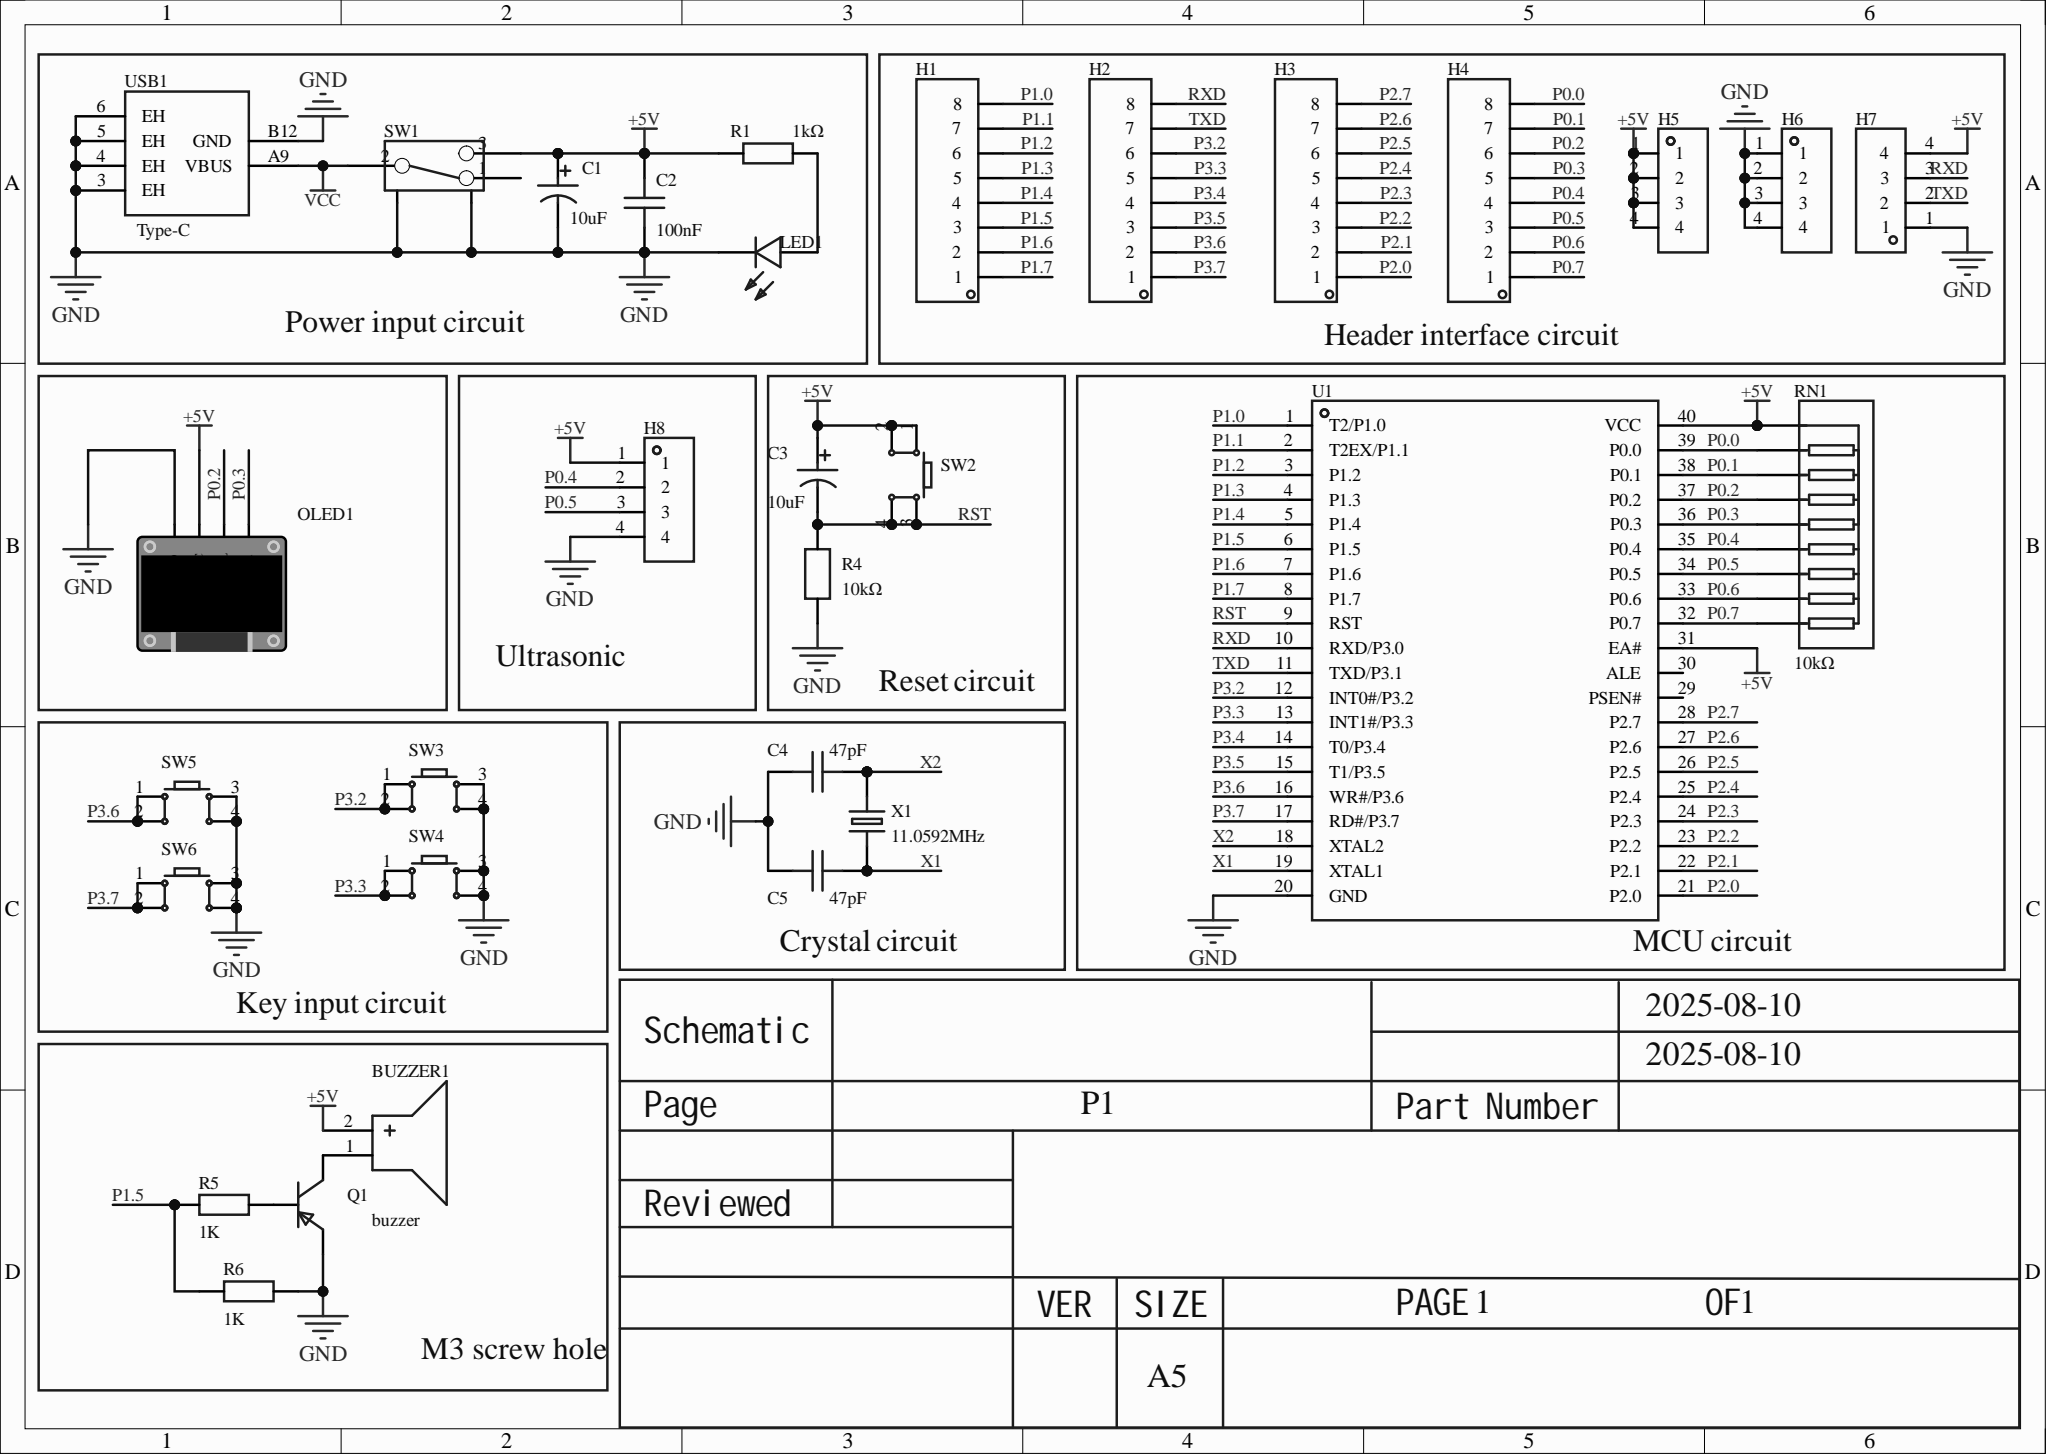Circuit board | Altium Designer | 47 parts | 49 nets
Bill of materials:
Comment,Description,Designator,Footprint,LibRef,Quantity
"buzzer","","BUZZER1","BUZ-TH_BD12.0-P6.00-D0.9-RD","buzzer","1"
"10uF","Capacitance: 10uF; Tolerance: ±20%; Rated voltage: 50V; Body diameter: 5mm; Body length: 11mm; Lead pitch: 2mm; Operating life: 1000hrs@105℃;","C1, C3","CAP-TH_BD5.0-P2.00-D0.8-FD","KM106M050D11RR0VH2FP0","2"
"100nF","Capacitance: 100nF; Tolerance: ±10%; Rated voltage: 50V; Temperature coefficient: X7R;","C2","CAP-TH_L8.5-W5.0-P5.00-D1.2","CT4-0805B104K500F3","1"
"47pF","Capacitance: 47pF; Tolerance: ±5%; Rated voltage: 50V; Temperature coefficient: NP0; Lead pitch: 5.08mm; Body diameter: 4.7mm; Body thickness: 2.2mm;","C4, C5","CAP-TH_L4.5-W3.0-P5.00-D1.2","CC1H470JC74DCH4B10MN","2"
"","","H1, H2, H3, H4","HDR-TH_8P-P2.54-V-M","HDR-M_2.54_1x8P","4"
"","","H5, H6, H7","HDR-TH_4P-P2.54-V-M","HDR-M_2.54_1x4P","3"
"","","H8","HDR-TH_4P-P2.54-V-F","HDR-F_2.54_1x4P","1"
"204-10SURD/S530-A3-L","Emitted color: Red; Diode configuration: -; Lens color: Diffused red; Dominant wavelength: 624nm; Peak wavelength: 632nm; Color temperature: -; Test current: 20mA; Power: 60mW; Viewing angle: 40°; Mounting style: -; Operating temperature: -40℃~+85℃;","LED1","LED-TH_BD3.0-P2.54-FD","204-10SURD/S530-A3-L","1"
"204-10SYGD/S530-E3","Emitted color: Green/Yellow-green;","LED2, LED3, LED4, LED5, LED6, LED7, LED8, LED9","LED-TH_BD3.8-P2.54-FD","204-10SYGD/S530-E3","8"
"","","OLED1","0.96OLED_4P","0.96OLED模块_4P","1"
"","","Q1","S8550P_SOT","S8550_SOT_PNP","1"
"1kΩ","Resistor type: Metal film resistor; Resistance: 1kΩ; Tolerance: ±1%; Power: 250mW; Temperature coefficient: ±50ppm/?;","R1, R2, R3, R7, R8, R9, R10, R11, R12","RES-TH_BD2.5-L6.5-P10.50-D0.6","MFR0W4F1001A50","9"
"10kΩ","","R4","RES-TH_BD2.4-L6.3-P10.30-D0.6","RN1/4W10KFT/BA1","1"
"1K","","R5, R6","R0603","Res_0603","2"
"10kΩ","Resistance: 10kΩ; Tolerance: ±5%; Power per element: 125mW; Temperature coefficient: ±100ppm/?; Resistor count: 8; Pin count: 9;","RN1","RES-ARRAY-TH_9P-P2.54-D1.0","A09-103JP","1"
"SS-12D02-VG4","Rated current (DC): -; Rated voltage (DC): -; Rated current (AC): -; Rated voltage (AC): -; Circuit configuration: SPDT; Mounting style: Through-hole; Mechanical life: 5000; Actuator shape: Rectangular post; Pin style: PC pin; Operating temperature: -25℃~+70℃; Switch height: 8.7mm;","SW1","SW-TH_SS-12D02-VG4","SS-12D02-VG4_C136719","1"
"","","SW2, SW3, SW4, SW5, SW6","SW-TH_4P-L6.0-W6.0-P4.50-LS6.5","Key_TH_6x6x6","5"
"STC89C52RC-40I-PDIP40","CPU core: 51 series; Max CPU frequency: -; Operating voltage: 3.3V~5.5V; Internal oscillator: -; External clock frequency range: -; Program FLASH size: 8KB; Total RAM: 512Byte; EEPROM/data FLASH size: 4KB; GPIO count: 35; ADC (units/channels/bits): -; DAC (units/channels/bits): -; (E)PWM (units/channels/bits): -; 8-bit Timer count: -; 16-bit Timer count: 3; 32-bit Timer count: -; Internal comparator count: -; U(S)ART count: 1; I2C count: -; I2S count: -;","U1","DIP-40_L52.0-W13.7-P2.54-LS15.2-BL","STC89C52RC-40I-PDIP40","1"
"TYPE-C-31-M-33","Connector type: Type-C; Standard: -; Gender: Female; Contact count: 2; Port count: 1; Mounting style: Right angle; Rated current - power: 3A; Operating temperature range: -30℃~+80℃;","USB1","USB-C-TH_TYPE-C-31-M-33","TYPE-C-31-M-33","1"
"11.059MHz","Crystal type: 49S crystal; Frequency: 11.059MHz; Frequency tolerance: ±30ppm; Frequency stability: ±30ppm; Load capacitance: 20pF; ESR: 50Ω; Operating temperature: -;","X1","HC-49US_L11.5-W4.5-P4.88","TAXD11.059M2GLFBET2T","1"
Netlist (Protel format):
[
BUZZER1
BUZ-TH_BD12.0-P6.00-D0.9-RD
buzzer



]
[
C1
CAP-TH_BD5.0-P2.00-D0.8-FD
10uF



]
[
C2
CAP-TH_L8.5-W5.0-P5.00-D1.2
100nF



]
[
C3
CAP-TH_BD5.0-P2.00-D0.8-FD
10uF



]
[
C4
CAP-TH_L4.5-W3.0-P5.00-D1.2
47pF



]
[
C5
CAP-TH_L4.5-W3.0-P5.00-D1.2
47pF



]
[
H1
HDR-TH_8P-P2.54-V-M




]
[
H2
HDR-TH_8P-P2.54-V-M




]
[
H3
HDR-TH_8P-P2.54-V-M




]
[
H4
HDR-TH_8P-P2.54-V-M




]
[
H5
HDR-TH_4P-P2.54-V-M




]
[
H6
HDR-TH_4P-P2.54-V-M




]
[
H7
HDR-TH_4P-P2.54-V-M




]
[
H8
HDR-TH_4P-P2.54-V-F




]
[
LED1
LED-TH_BD3.0-P2.54-FD
204-10SURD/S530-A3-L



]
[
LED2
LED-TH_BD3.8-P2.54-FD
204-10SYGD/S530-E3



]
[
LED3
LED-TH_BD3.8-P2.54-FD
204-10SYGD/S530-E3



]
[
LED4
LED-TH_BD3.8-P2.54-FD
204-10SYGD/S530-E3



]
[
LED5
LED-TH_BD3.8-P2.54-FD
204-10SYGD/S530-E3



]
[
LED6
LED-TH_BD3.8-P2.54-FD
204-10SYGD/S530-E3



]
[
LED7
LED-TH_BD3.8-P2.54-FD
204-10SYGD/S530-E3



]
[
LED8
LED-TH_BD3.8-P2.54-FD
204-10SYGD/S530-E3



]
[
LED9
LED-TH_BD3.8-P2.54-FD
204-10SYGD/S530-E3



]
[
OLED1
0.96OLED_4P




]
[
Q1
S8550P_SOT




]
[
R1
RES-TH_BD2.5-L6.5-P10.50-D0.6
1kΩ



]
[
R2
RES-TH_BD2.5-L6.5-P10.50-D0.6
1kΩ



]
[
R3
RES-TH_BD2.5-L6.5-P10.50-D0.6
1kΩ



]
[
R4
RES-TH_BD2.4-L6.3-P10.30-D0.6
10kΩ



]
[
R5
R0603
1K



]
[
R6
R0603
1K



]
[
R7
RES-TH_BD2.5-L6.5-P10.50-D0.6
1kΩ



]
[
R8
RES-TH_BD2.5-L6.5-P10.50-D0.6
1kΩ



]
[
R9
RES-TH_BD2.5-L6.5-P10.50-D0.6
1kΩ



]
[
R10
RES-TH_BD2.5-L6.5-P10.50-D0.6
1kΩ



]
[
R11
RES-TH_BD2.5-L6.5-P10.50-D0.6
1kΩ



]
[
R12
RES-TH_BD2.5-L6.5-P10.50-D0.6
1kΩ



]
[
RN1
RES-ARRAY-TH_9P-P2.54-D1.0
10kΩ



]
[
SW1
SW-TH_SS-12D02-VG4
SS-12D02-VG4



]
[
SW2
SW-TH_4P-L6.0-W6.0-P4.50-LS6.5




]
[
SW3
SW-TH_4P-L6.0-W6.0-P4.50-LS6.5




]
[
SW4
SW-TH_4P-L6.0-W6.0-P4.50-LS6.5




]
[
SW5
SW-TH_4P-L6.0-W6.0-P4.50-LS6.5




]
[
SW6
SW-TH_4P-L6.0-W6.0-P4.50-LS6.5




]
[
U1
DIP-40_L52.0-W13.7-P2.54-LS15.2-BL
STC89C52RC-40I-PDIP40



]
[
USB1
USB-C-TH_TYPE-C-31-M-33
TYPE-C-31-M-33



]
[
X1
HC-49US_L11.5-W4.5-P4.88
11.0592MHz



]
(
X2
C4-2
U1-18
X1-2
)
(
X1
C5-2
U1-19
X1-1
)
(
VCC
SW1-2
USB1-A9
)
(
TXD
H2-7
H7-2
U1-11
)
(
RXD
H2-8
H7-3
U1-10
)
(
RST
C3-2
R4-2
SW2-3
SW2-4
U1-9
)
(
P3.7
H2-1
SW6-1
SW6-2
U1-17
)
(
P3.6
H2-2
SW5-1
SW5-2
U1-16
)
(
P3.5
H2-3
U1-15
)
(
P3.4
H2-4
U1-14
)
(
P3.3
H2-5
SW4-1
SW4-2
U1-13
)
(
P3.2
H2-6
SW3-1
SW3-2
U1-12
)
(
P2.7
H3-8
LED9-2
U1-28
)
(
P2.6
H3-7
LED8-2
U1-27
)
(
P2.5
H3-6
LED7-2
U1-26
)
(
P2.4
H3-5
LED6-2
U1-25
)
(
P2.3
H3-4
LED5-2
U1-24
)
(
P2.2
H3-3
LED4-2
U1-23
)
(
P2.1
H3-2
LED3-2
U1-22
)
(
P2.0
H3-1
LED2-2
U1-21
)
(
P1.7
H1-1
U1-8
)
(
P1.6
H1-2
U1-7
)
(
P1.5
H1-3
R5-1
R6-1
U1-6
)
(
P1.4
H1-4
U1-5
)
(
P1.3
H1-5
U1-4
)
(
P1.2
H1-6
U1-3
)
(
P1.1
H1-7
U1-2
)
(
P1.0
H1-8
U1-1
)
(
P0.7
H4-1
RN1-9
U1-32
)
(
P0.6
H4-2
RN1-8
U1-33
)
(
P0.5
H4-3
H8-3
RN1-7
U1-34
)
(
P0.4
H4-4
H8-2
RN1-6
U1-35
)
(
P0.3
H4-5
OLED1-4
RN1-5
U1-36
)
(
P0.2
H4-6
OLED1-3
RN1-4
U1-37
)
(
P0.1
H4-7
RN1-3
U1-38
)
(
P0.0
H4-8
RN1-2
U1-39
)
(
NetQ1_1
Q1-1
R5-2
)
(
NetLED9_1
LED9-1
R12-2
)
(
NetLED8_1
LED8-1
R11-2
)
(
NetLED7_1
LED7-1
R10-2
)
(
NetLED6_1
LED6-1
R9-2
)
(
NetLED5_1
LED5-1
R8-2
)
(
NetLED4_1
LED4-1
R7-2
)
(
NetLED3_1
LED3-1
R3-2
)
(
NetLED2_1
LED2-1
R2-2
)
(
NetLED1_1
LED1-1
R1-2
)
(
NetBUZZER1_1
BUZZER1-1
Q1-3
)
(
GND
C1-2
C2-1
C4-1
C5-1
H6-1
H6-2
H6-3
H6-4
H7-1
H8-4
LED1-2
OLED1-1
Q1-2
R4-1
R6-2
SW1-4
SW1-5
SW3-3
SW3-4
SW4-3
SW4-4
SW5-3
SW5-4
SW6-3
SW6-4
U1-20
USB1-3
USB1-4
USB1-5
USB1-6
USB1-B12
)
(
+5V
BUZZER1-2
C1-1
C2-2
C3-1
H5-1
H5-2
H5-3
H5-4
H7-4
H8-1
OLED1-2
R1-1
R2-1
R3-1
R7-1
R8-1
R9-1
R10-1
R11-1
R12-1
RN1-1
SW1-3
SW2-1
SW2-2
U1-31
U1-40
)